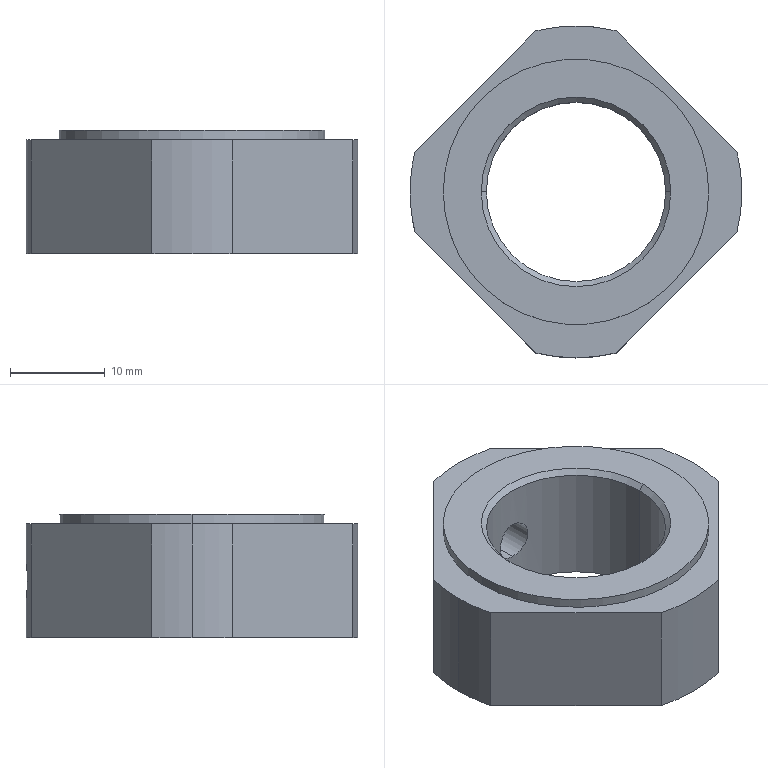Part | STEP file | BKN26-M20 | 1 solid | 20 faces | box 35 x 35 x 13 mm | volume 6926 mm3 | cylinder 11 | plane 7 | cone 2 | commonest cylinder face diameters 35 x5 4.134 x2 18.917 x2 28 x2
STEP:
#1=CARTESIAN_POINT('',(9.458,0.,12.459));
#2=VERTEX_POINT('',#1);
#3=CARTESIAN_POINT('',(-9.458,0.,12.459));
#4=VERTEX_POINT('',#3);
#5=CARTESIAN_POINT('',(0.,0.,12.459));
#6=DIRECTION('',(0.,0.,-1.));
#7=DIRECTION('',(-1.,0.,0.));
#8=AXIS2_PLACEMENT_3D('',#5,#6,#7);
#9=CIRCLE('',#8,9.458);
#10=EDGE_CURVE('',#2,#4,#9,.T.);
#11=ORIENTED_EDGE('',*,*,#10,.T.);
#12=CARTESIAN_POINT('',(-10.,0.,13.));
#13=VERTEX_POINT('',#12);
#14=CARTESIAN_POINT('',(-10.,0.,13.));
#15=DIRECTION('',(-0.7071,0.,0.7071));
#16=VECTOR('',#15,1000.);
#17=LINE('',#14,#16);
#18=EDGE_CURVE('',#4,#13,#17,.T.);
#19=ORIENTED_EDGE('',*,*,#18,.T.);
#20=CARTESIAN_POINT('',(10.,0.,13.));
#21=VERTEX_POINT('',#20);
#22=CARTESIAN_POINT('',(0.,0.,13.));
#23=DIRECTION('',(0.,0.,-1.));
#24=DIRECTION('',(-1.,0.,0.));
#25=AXIS2_PLACEMENT_3D('',#22,#23,#24);
#26=CIRCLE('',#25,10.);
#27=EDGE_CURVE('',#21,#13,#26,.T.);
#28=ORIENTED_EDGE('',*,*,#27,.F.);
#29=CARTESIAN_POINT('',(10.,0.,13.));
#30=DIRECTION('',(0.7071,0.,0.7071));
#31=VECTOR('',#30,1000.);
#32=LINE('',#29,#31);
#33=EDGE_CURVE('',#2,#21,#32,.T.);
#34=ORIENTED_EDGE('',*,*,#33,.F.);
#35=EDGE_LOOP('',(#11,#19,#28,#34));
#36=FACE_OUTER_BOUND('',#35,.T.);
#37=CARTESIAN_POINT('',(0.,0.,13.));
#38=DIRECTION('',(0.,0.,1.));
#39=DIRECTION('',(1.,0.,0.));
#40=AXIS2_PLACEMENT_3D('',#37,#38,#39);
#41=CONICAL_SURFACE('',#40,10.,0.7854);
#42=ADVANCED_FACE('',(#36),#41,.F.);
#43=CARTESIAN_POINT('',(14.,0.,13.));
#44=VERTEX_POINT('',#43);
#45=CARTESIAN_POINT('',(-14.,0.,13.));
#46=VERTEX_POINT('',#45);
#47=CARTESIAN_POINT('',(0.,0.,13.));
#48=DIRECTION('',(0.,0.,1.));
#49=DIRECTION('',(1.,0.,0.));
#50=AXIS2_PLACEMENT_3D('',#47,#48,#49);
#51=CIRCLE('',#50,14.);
#52=EDGE_CURVE('',#44,#46,#51,.T.);
#53=ORIENTED_EDGE('',*,*,#52,.F.);
#54=CARTESIAN_POINT('',(14.,0.,12.));
#55=VERTEX_POINT('',#54);
#56=CARTESIAN_POINT('',(14.,0.,13.));
#57=DIRECTION('',(0.,0.,-1.));
#58=VECTOR('',#57,1000.);
#59=LINE('',#56,#58);
#60=EDGE_CURVE('',#44,#55,#59,.T.);
#61=ORIENTED_EDGE('',*,*,#60,.T.);
#62=CARTESIAN_POINT('',(-14.,0.,12.));
#63=VERTEX_POINT('',#62);
#64=CARTESIAN_POINT('',(0.,0.,12.));
#65=DIRECTION('',(0.,0.,-1.));
#66=DIRECTION('',(1.,0.,0.));
#67=AXIS2_PLACEMENT_3D('',#64,#65,#66);
#68=CIRCLE('',#67,14.);
#69=EDGE_CURVE('',#63,#55,#68,.T.);
#70=ORIENTED_EDGE('',*,*,#69,.F.);
#71=CARTESIAN_POINT('',(-14.,0.,13.));
#72=DIRECTION('',(0.,0.,-1.));
#73=VECTOR('',#72,1000.);
#74=LINE('',#71,#73);
#75=EDGE_CURVE('',#46,#63,#74,.T.);
#76=ORIENTED_EDGE('',*,*,#75,.F.);
#77=EDGE_LOOP('',(#53,#61,#70,#76));
#78=FACE_OUTER_BOUND('',#77,.T.);
#79=CARTESIAN_POINT('',(0.,0.,13.));
#80=DIRECTION('',(0.,0.,-1.));
#81=DIRECTION('',(-1.,0.,0.));
#82=AXIS2_PLACEMENT_3D('',#79,#80,#81);
#83=CYLINDRICAL_SURFACE('',#82,14.);
#84=ADVANCED_FACE('',(#78),#83,.T.);
#85=CARTESIAN_POINT('',(-17.5,0.,12.));
#86=VERTEX_POINT('',#85);
#87=CARTESIAN_POINT('',(-16.98,-4.233,12.));
#88=VERTEX_POINT('',#87);
#89=CARTESIAN_POINT('',(0.,0.,12.));
#90=DIRECTION('',(0.,0.,1.));
#91=DIRECTION('',(-0.9703,0.2419,0.));
#92=AXIS2_PLACEMENT_3D('',#89,#90,#91);
#93=CIRCLE('',#92,17.5);
#94=EDGE_CURVE('',#86,#88,#93,.T.);
#95=ORIENTED_EDGE('',*,*,#94,.F.);
#96=CARTESIAN_POINT('',(-17.5,0.,0.));
#97=VERTEX_POINT('',#96);
#98=CARTESIAN_POINT('',(-17.5,0.,12.));
#99=DIRECTION('',(0.,0.,-1.));
#100=VECTOR('',#99,1000.);
#101=LINE('',#98,#100);
#102=EDGE_CURVE('',#86,#97,#101,.T.);
#103=ORIENTED_EDGE('',*,*,#102,.T.);
#104=CARTESIAN_POINT('',(-16.98,-4.233,0.));
#105=VERTEX_POINT('',#104);
#106=CARTESIAN_POINT('',(0.,0.,0.));
#107=DIRECTION('',(0.,0.,1.));
#108=DIRECTION('',(-0.9703,0.2419,0.));
#109=AXIS2_PLACEMENT_3D('',#106,#107,#108);
#110=CIRCLE('',#109,17.5);
#111=EDGE_CURVE('',#97,#105,#110,.T.);
#112=ORIENTED_EDGE('',*,*,#111,.T.);
#113=CARTESIAN_POINT('',(-16.98,-4.233,12.));
#114=DIRECTION('',(0.,0.,-1.));
#115=VECTOR('',#114,1000.);
#116=LINE('',#113,#115);
#117=EDGE_CURVE('',#88,#105,#116,.T.);
#118=ORIENTED_EDGE('',*,*,#117,.F.);
#119=EDGE_LOOP('',(#95,#103,#112,#118));
#120=FACE_OUTER_BOUND('',#119,.T.);
#121=CARTESIAN_POINT('',(0.,0.,12.));
#122=DIRECTION('',(0.,0.,-1.));
#123=DIRECTION('',(-1.,0.,0.));
#124=AXIS2_PLACEMENT_3D('',#121,#122,#123);
#125=CYLINDRICAL_SURFACE('',#124,17.5);
#126=ADVANCED_FACE('',(#120),#125,.T.);
#127=ORIENTED_EDGE('',*,*,#10,.F.);
#128=CARTESIAN_POINT('',(9.458,0.,0.));
#129=VERTEX_POINT('',#128);
#130=CARTESIAN_POINT('',(9.458,0.,0.));
#131=DIRECTION('',(0.,0.,-1.));
#132=VECTOR('',#131,1000.);
#133=LINE('',#130,#132);
#134=EDGE_CURVE('',#2,#129,#133,.T.);
#135=ORIENTED_EDGE('',*,*,#134,.T.);
#136=CARTESIAN_POINT('',(-9.458,0.,0.));
#137=VERTEX_POINT('',#136);
#138=CARTESIAN_POINT('',(0.,0.,0.));
#139=DIRECTION('',(0.,0.,-1.));
#140=DIRECTION('',(-1.,0.,0.));
#141=AXIS2_PLACEMENT_3D('',#138,#139,#140);
#142=CIRCLE('',#141,9.458);
#143=EDGE_CURVE('',#129,#137,#142,.T.);
#144=ORIENTED_EDGE('',*,*,#143,.T.);
#145=CARTESIAN_POINT('',(-9.458,0.,0.));
#146=DIRECTION('',(0.,0.,-1.));
#147=VECTOR('',#146,1000.);
#148=LINE('',#145,#147);
#149=EDGE_CURVE('',#4,#137,#148,.T.);
#150=ORIENTED_EDGE('',*,*,#149,.F.);
#151=EDGE_LOOP('',(#127,#135,#144,#150));
#152=FACE_OUTER_BOUND('',#151,.T.);
#153=CARTESIAN_POINT('',(0.,0.,0.));
#154=DIRECTION('',(0.,0.,-1.));
#155=DIRECTION('',(-1.,0.,0.));
#156=AXIS2_PLACEMENT_3D('',#153,#154,#155);
#157=CYLINDRICAL_SURFACE('',#156,9.458);
#158=ADVANCED_FACE('',(#152),#157,.F.);
#159=CARTESIAN_POINT('',(0.,17.5,3.933));
#160=VERTEX_POINT('',#159);
#161=CARTESIAN_POINT('',(-0.000000115,17.5,8.067));
#162=VERTEX_POINT('',#161);
#163=CARTESIAN_POINT('',(0.,17.5,3.933));
#164=CARTESIAN_POINT('',(-0.2708,17.5,3.933));
#165=CARTESIAN_POINT('',(-0.5415,17.493,3.987));
#166=CARTESIAN_POINT('',(-1.041,17.471,4.194));
#167=CARTESIAN_POINT('',(-1.27,17.455,4.347));
#168=CARTESIAN_POINT('',(-1.653,17.423,4.73));
#169=CARTESIAN_POINT('',(-1.806,17.407,4.959));
#170=CARTESIAN_POINT('',(-2.013,17.384,5.459));
#171=CARTESIAN_POINT('',(-2.067,17.378,5.729));
#172=CARTESIAN_POINT('',(-2.067,17.377,6.271));
#173=CARTESIAN_POINT('',(-2.013,17.384,6.541));
#174=CARTESIAN_POINT('',(-1.806,17.407,7.041));
#175=CARTESIAN_POINT('',(-1.653,17.423,7.27));
#176=CARTESIAN_POINT('',(-1.27,17.455,7.653));
#177=CARTESIAN_POINT('',(-1.041,17.471,7.806));
#178=CARTESIAN_POINT('',(-0.5414,17.493,8.013));
#179=CARTESIAN_POINT('',(-0.2708,17.5,8.067));
#180=CARTESIAN_POINT('',(-0.000000115,17.5,8.067));
#181=B_SPLINE_CURVE_WITH_KNOTS('',3,(#163,#164,#165,#166,#167,#168,#169,#170,#171,#172,#173,#174,#175,#176,#177,#178,#179,#180),.UNSPECIFIED.,.F.,.F.,(4,2,2,2,2,2,2,2,4),(0.,0.8086,1.617,2.426,3.234,4.043,4.851,5.66,6.469),.UNSPECIFIED.);
#182=EDGE_CURVE('',#160,#162,#181,.T.);
#183=ORIENTED_EDGE('',*,*,#182,.T.);
#184=CARTESIAN_POINT('',(-0.000000086,9.458,8.067));
#185=VERTEX_POINT('',#184);
#186=CARTESIAN_POINT('',(0.,9.,8.067));
#187=DIRECTION('',(0.,-1.,0.));
#188=VECTOR('',#187,1000.);
#189=LINE('',#186,#188);
#190=EDGE_CURVE('',#162,#185,#189,.T.);
#191=ORIENTED_EDGE('',*,*,#190,.T.);
#192=CARTESIAN_POINT('',(0.,9.458,3.933));
#193=VERTEX_POINT('',#192);
#194=CARTESIAN_POINT('',(0.,9.458,3.933));
#195=CARTESIAN_POINT('',(-0.137,9.458,3.933));
#196=CARTESIAN_POINT('',(-0.2717,9.456,3.946));
#197=CARTESIAN_POINT('',(-0.5365,9.444,3.999));
#198=CARTESIAN_POINT('',(-0.6679,9.436,4.039));
#199=CARTESIAN_POINT('',(-0.9182,9.415,4.143));
#200=CARTESIAN_POINT('',(-1.037,9.402,4.206));
#201=CARTESIAN_POINT('',(-1.261,9.375,4.357));
#202=CARTESIAN_POINT('',(-1.367,9.36,4.444));
#203=CARTESIAN_POINT('',(-1.652,9.315,4.729));
#204=CARTESIAN_POINT('',(-1.806,9.285,4.959));
#205=CARTESIAN_POINT('',(-2.012,9.243,5.456));
#206=CARTESIAN_POINT('',(-2.067,9.23,5.729));
#207=CARTESIAN_POINT('',(-2.067,9.23,6.134));
#208=CARTESIAN_POINT('',(-2.054,9.233,6.272));
#209=CARTESIAN_POINT('',(-2.001,9.245,6.537));
#210=CARTESIAN_POINT('',(-1.961,9.253,6.666));
#211=CARTESIAN_POINT('',(-1.805,9.285,7.043));
#212=CARTESIAN_POINT('',(-1.653,9.315,7.27));
#213=CARTESIAN_POINT('',(-1.365,9.36,7.558));
#214=CARTESIAN_POINT('',(-1.262,9.375,7.643));
#215=CARTESIAN_POINT('',(-1.038,9.402,7.793));
#216=CARTESIAN_POINT('',(-0.9169,9.415,7.857));
#217=CARTESIAN_POINT('',(-0.6672,9.436,7.961));
#218=CARTESIAN_POINT('',(-0.5383,9.444,8.001));
#219=CARTESIAN_POINT('',(-0.2723,9.456,8.053));
#220=CARTESIAN_POINT('',(-0.1352,9.458,8.067));
#221=CARTESIAN_POINT('',(-0.000000086,9.458,8.067));
#222=B_SPLINE_CURVE_WITH_KNOTS('',3,(#194,#195,#196,#197,#198,#199,#200,#201,#202,#203,#204,#205,#206,#207,#208,#209,#210,#211,#212,#213,#214,#215,#216,#217,#218,#219,#220,#221),.UNSPECIFIED.,.F.,.F.,(4,2,2,2,2,2,2,2,2,2,2,2,2,4),(0.,0.4051,0.8102,1.215,1.62,2.431,3.241,3.646,4.051,4.861,5.267,5.672,6.077,6.482),.UNSPECIFIED.);
#223=EDGE_CURVE('',#193,#185,#222,.T.);
#224=ORIENTED_EDGE('',*,*,#223,.F.);
#225=CARTESIAN_POINT('',(0.,9.,3.933));
#226=DIRECTION('',(0.,-1.,0.));
#227=VECTOR('',#226,1000.);
#228=LINE('',#225,#227);
#229=EDGE_CURVE('',#160,#193,#228,.T.);
#230=ORIENTED_EDGE('',*,*,#229,.F.);
#231=EDGE_LOOP('',(#183,#191,#224,#230));
#232=FACE_OUTER_BOUND('',#231,.T.);
#233=CARTESIAN_POINT('',(0.,9.,6.));
#234=DIRECTION('',(0.,-1.,0.));
#235=DIRECTION('',(0.,0.,-1.));
#236=AXIS2_PLACEMENT_3D('',#233,#234,#235);
#237=CYLINDRICAL_SURFACE('',#236,2.067);
#238=ADVANCED_FACE('',(#232),#237,.F.);
#239=CARTESIAN_POINT('',(4.233,16.98,0.));
#240=VERTEX_POINT('',#239);
#241=CARTESIAN_POINT('',(-4.233,16.98,0.));
#242=VERTEX_POINT('',#241);
#243=CARTESIAN_POINT('',(0.,0.,0.));
#244=DIRECTION('',(0.,0.,1.));
#245=DIRECTION('',(0.2419,0.9703,0.));
#246=AXIS2_PLACEMENT_3D('',#243,#244,#245);
#247=CIRCLE('',#246,17.5);
#248=EDGE_CURVE('',#240,#242,#247,.T.);
#249=ORIENTED_EDGE('',*,*,#248,.T.);
#250=CARTESIAN_POINT('',(-4.233,16.98,12.));
#251=VERTEX_POINT('',#250);
#252=CARTESIAN_POINT('',(-4.233,16.98,12.));
#253=DIRECTION('',(0.,0.,-1.));
#254=VECTOR('',#253,1000.);
#255=LINE('',#252,#254);
#256=EDGE_CURVE('',#251,#242,#255,.T.);
#257=ORIENTED_EDGE('',*,*,#256,.F.);
#258=CARTESIAN_POINT('',(4.233,16.98,12.));
#259=VERTEX_POINT('',#258);
#260=CARTESIAN_POINT('',(0.,0.,12.));
#261=DIRECTION('',(0.,0.,1.));
#262=DIRECTION('',(0.2419,0.9703,0.));
#263=AXIS2_PLACEMENT_3D('',#260,#261,#262);
#264=CIRCLE('',#263,17.5);
#265=EDGE_CURVE('',#259,#251,#264,.T.);
#266=ORIENTED_EDGE('',*,*,#265,.F.);
#267=CARTESIAN_POINT('',(4.233,16.98,12.));
#268=DIRECTION('',(0.,0.,-1.));
#269=VECTOR('',#268,1000.);
#270=LINE('',#267,#269);
#271=EDGE_CURVE('',#259,#240,#270,.T.);
#272=ORIENTED_EDGE('',*,*,#271,.T.);
#273=EDGE_LOOP('',(#249,#257,#266,#272));
#274=FACE_OUTER_BOUND('',#273,.T.);
#275=ORIENTED_EDGE('',*,*,#182,.F.);
#276=CARTESIAN_POINT('',(-0.000000115,17.5,8.067));
#277=CARTESIAN_POINT('',(0.2707,17.5,8.067));
#278=CARTESIAN_POINT('',(0.5413,17.493,8.013));
#279=CARTESIAN_POINT('',(1.041,17.471,7.806));
#280=CARTESIAN_POINT('',(1.27,17.455,7.653));
#281=CARTESIAN_POINT('',(1.652,17.423,7.271));
#282=CARTESIAN_POINT('',(1.805,17.407,7.042));
#283=CARTESIAN_POINT('',(2.013,17.384,6.542));
#284=CARTESIAN_POINT('',(2.067,17.378,6.272));
#285=CARTESIAN_POINT('',(2.067,17.377,5.731));
#286=CARTESIAN_POINT('',(2.013,17.384,5.46));
#287=CARTESIAN_POINT('',(1.807,17.407,4.96));
#288=CARTESIAN_POINT('',(1.654,17.423,4.731));
#289=CARTESIAN_POINT('',(1.272,17.455,4.348));
#290=CARTESIAN_POINT('',(1.043,17.471,4.195));
#291=CARTESIAN_POINT('',(0.5441,17.493,3.988));
#292=CARTESIAN_POINT('',(0.2722,17.5,3.933));
#293=CARTESIAN_POINT('',(0.,17.5,3.933));
#294=B_SPLINE_CURVE_WITH_KNOTS('',3,(#276,#277,#278,#279,#280,#281,#282,#283,#284,#285,#286,#287,#288,#289,#290,#291,#292,#293),.UNSPECIFIED.,.F.,.F.,(4,2,2,2,2,2,2,2,4),(6.469,7.277,8.085,8.893,9.702,10.51,11.318,12.126,12.935),.UNSPECIFIED.);
#295=EDGE_CURVE('',#162,#160,#294,.T.);
#296=ORIENTED_EDGE('',*,*,#295,.F.);
#297=EDGE_LOOP('',(#275,#296));
#298=FACE_BOUND('',#297,.T.);
#299=CARTESIAN_POINT('',(0.,0.,12.));
#300=DIRECTION('',(0.,0.,-1.));
#301=DIRECTION('',(-1.,0.,0.));
#302=AXIS2_PLACEMENT_3D('',#299,#300,#301);
#303=CYLINDRICAL_SURFACE('',#302,17.5);
#304=ADVANCED_FACE('',(#274,#298),#303,.T.);
#305=CARTESIAN_POINT('',(0.,0.,0.));
#306=DIRECTION('',(0.,0.,-1.));
#307=DIRECTION('',(-1.,0.,0.));
#308=AXIS2_PLACEMENT_3D('',#305,#306,#307);
#309=CIRCLE('',#308,9.458);
#310=EDGE_CURVE('',#137,#129,#309,.T.);
#311=ORIENTED_EDGE('',*,*,#310,.F.);
#312=ORIENTED_EDGE('',*,*,#143,.F.);
#313=EDGE_LOOP('',(#311,#312));
#314=FACE_BOUND('',#313,.T.);
#315=CARTESIAN_POINT('',(-16.98,4.233,0.));
#316=VERTEX_POINT('',#315);
#317=CARTESIAN_POINT('',(-4.233,16.98,0.));
#318=DIRECTION('',(-0.7071,-0.7071,0.));
#319=VECTOR('',#318,1000.);
#320=LINE('',#317,#319);
#321=EDGE_CURVE('',#242,#316,#320,.T.);
#322=ORIENTED_EDGE('',*,*,#321,.F.);
#323=ORIENTED_EDGE('',*,*,#248,.F.);
#324=CARTESIAN_POINT('',(16.98,4.233,0.));
#325=VERTEX_POINT('',#324);
#326=CARTESIAN_POINT('',(16.98,4.233,0.));
#327=DIRECTION('',(-0.7071,0.7071,0.));
#328=VECTOR('',#327,1000.);
#329=LINE('',#326,#328);
#330=EDGE_CURVE('',#325,#240,#329,.T.);
#331=ORIENTED_EDGE('',*,*,#330,.F.);
#332=CARTESIAN_POINT('',(16.98,-4.233,0.));
#333=VERTEX_POINT('',#332);
#334=CARTESIAN_POINT('',(0.,0.,0.));
#335=DIRECTION('',(0.,0.,1.));
#336=DIRECTION('',(0.9703,-0.2419,0.));
#337=AXIS2_PLACEMENT_3D('',#334,#335,#336);
#338=CIRCLE('',#337,17.5);
#339=EDGE_CURVE('',#333,#325,#338,.T.);
#340=ORIENTED_EDGE('',*,*,#339,.F.);
#341=CARTESIAN_POINT('',(4.233,-16.98,0.));
#342=VERTEX_POINT('',#341);
#343=CARTESIAN_POINT('',(4.233,-16.98,0.));
#344=DIRECTION('',(0.7071,0.7071,0.));
#345=VECTOR('',#344,1000.);
#346=LINE('',#343,#345);
#347=EDGE_CURVE('',#342,#333,#346,.T.);
#348=ORIENTED_EDGE('',*,*,#347,.F.);
#349=CARTESIAN_POINT('',(-4.233,-16.98,0.));
#350=VERTEX_POINT('',#349);
#351=CARTESIAN_POINT('',(0.,0.,0.));
#352=DIRECTION('',(0.,0.,1.));
#353=DIRECTION('',(-0.2419,-0.9703,0.));
#354=AXIS2_PLACEMENT_3D('',#351,#352,#353);
#355=CIRCLE('',#354,17.5);
#356=EDGE_CURVE('',#350,#342,#355,.T.);
#357=ORIENTED_EDGE('',*,*,#356,.F.);
#358=CARTESIAN_POINT('',(-16.98,-4.233,0.));
#359=DIRECTION('',(0.7071,-0.7071,0.));
#360=VECTOR('',#359,1000.);
#361=LINE('',#358,#360);
#362=EDGE_CURVE('',#105,#350,#361,.T.);
#363=ORIENTED_EDGE('',*,*,#362,.F.);
#364=ORIENTED_EDGE('',*,*,#111,.F.);
#365=CARTESIAN_POINT('',(0.,0.,0.));
#366=DIRECTION('',(0.,0.,1.));
#367=DIRECTION('',(-0.9703,0.2419,0.));
#368=AXIS2_PLACEMENT_3D('',#365,#366,#367);
#369=CIRCLE('',#368,17.5);
#370=EDGE_CURVE('',#316,#97,#369,.T.);
#371=ORIENTED_EDGE('',*,*,#370,.F.);
#372=EDGE_LOOP('',(#322,#323,#331,#340,#348,#357,#363,#364,#371));
#373=FACE_OUTER_BOUND('',#372,.T.);
#374=CARTESIAN_POINT('',(0.,0.,0.));
#375=DIRECTION('',(0.,0.,1.));
#376=DIRECTION('',(1.,0.,0.));
#377=AXIS2_PLACEMENT_3D('',#374,#375,#376);
#378=PLANE('',#377);
#379=ADVANCED_FACE('',(#314,#373),#378,.F.);
#380=ORIENTED_EDGE('',*,*,#321,.T.);
#381=CARTESIAN_POINT('',(-16.98,4.233,12.));
#382=VERTEX_POINT('',#381);
#383=CARTESIAN_POINT('',(-16.98,4.233,12.));
#384=DIRECTION('',(0.,0.,-1.));
#385=VECTOR('',#384,1000.);
#386=LINE('',#383,#385);
#387=EDGE_CURVE('',#382,#316,#386,.T.);
#388=ORIENTED_EDGE('',*,*,#387,.F.);
#389=CARTESIAN_POINT('',(-4.233,16.98,12.));
#390=DIRECTION('',(-0.7071,-0.7071,0.));
#391=VECTOR('',#390,1000.);
#392=LINE('',#389,#391);
#393=EDGE_CURVE('',#251,#382,#392,.T.);
#394=ORIENTED_EDGE('',*,*,#393,.F.);
#395=ORIENTED_EDGE('',*,*,#256,.T.);
#396=EDGE_LOOP('',(#380,#388,#394,#395));
#397=FACE_OUTER_BOUND('',#396,.T.);
#398=CARTESIAN_POINT('',(-4.233,16.98,12.));
#399=DIRECTION('',(0.7071,-0.7071,0.));
#400=DIRECTION('',(0.7071,0.7071,0.));
#401=AXIS2_PLACEMENT_3D('',#398,#399,#400);
#402=PLANE('',#401);
#403=ADVANCED_FACE('',(#397),#402,.F.);
#404=ORIENTED_EDGE('',*,*,#69,.T.);
#405=CARTESIAN_POINT('',(0.,0.,12.));
#406=DIRECTION('',(0.,0.,-1.));
#407=DIRECTION('',(1.,0.,0.));
#408=AXIS2_PLACEMENT_3D('',#405,#406,#407);
#409=CIRCLE('',#408,14.);
#410=EDGE_CURVE('',#55,#63,#409,.T.);
#411=ORIENTED_EDGE('',*,*,#410,.T.);
#412=EDGE_LOOP('',(#404,#411));
#413=FACE_BOUND('',#412,.T.);
#414=ORIENTED_EDGE('',*,*,#393,.T.);
#415=CARTESIAN_POINT('',(0.,0.,12.));
#416=DIRECTION('',(0.,0.,1.));
#417=DIRECTION('',(-0.9703,0.2419,0.));
#418=AXIS2_PLACEMENT_3D('',#415,#416,#417);
#419=CIRCLE('',#418,17.5);
#420=EDGE_CURVE('',#382,#86,#419,.T.);
#421=ORIENTED_EDGE('',*,*,#420,.T.);
#422=ORIENTED_EDGE('',*,*,#94,.T.);
#423=CARTESIAN_POINT('',(-4.233,-16.98,12.));
#424=VERTEX_POINT('',#423);
#425=CARTESIAN_POINT('',(-16.98,-4.233,12.));
#426=DIRECTION('',(0.7071,-0.7071,0.));
#427=VECTOR('',#426,1000.);
#428=LINE('',#425,#427);
#429=EDGE_CURVE('',#88,#424,#428,.T.);
#430=ORIENTED_EDGE('',*,*,#429,.T.);
#431=CARTESIAN_POINT('',(4.233,-16.98,12.));
#432=VERTEX_POINT('',#431);
#433=CARTESIAN_POINT('',(0.,0.,12.));
#434=DIRECTION('',(0.,0.,1.));
#435=DIRECTION('',(-0.2419,-0.9703,0.));
#436=AXIS2_PLACEMENT_3D('',#433,#434,#435);
#437=CIRCLE('',#436,17.5);
#438=EDGE_CURVE('',#424,#432,#437,.T.);
#439=ORIENTED_EDGE('',*,*,#438,.T.);
#440=CARTESIAN_POINT('',(16.98,-4.233,12.));
#441=VERTEX_POINT('',#440);
#442=CARTESIAN_POINT('',(4.233,-16.98,12.));
#443=DIRECTION('',(0.7071,0.7071,0.));
#444=VECTOR('',#443,1000.);
#445=LINE('',#442,#444);
#446=EDGE_CURVE('',#432,#441,#445,.T.);
#447=ORIENTED_EDGE('',*,*,#446,.T.);
#448=CARTESIAN_POINT('',(16.98,4.233,12.));
#449=VERTEX_POINT('',#448);
#450=CARTESIAN_POINT('',(0.,0.,12.));
#451=DIRECTION('',(0.,0.,1.));
#452=DIRECTION('',(0.9703,-0.2419,0.));
#453=AXIS2_PLACEMENT_3D('',#450,#451,#452);
#454=CIRCLE('',#453,17.5);
#455=EDGE_CURVE('',#441,#449,#454,.T.);
#456=ORIENTED_EDGE('',*,*,#455,.T.);
#457=CARTESIAN_POINT('',(16.98,4.233,12.));
#458=DIRECTION('',(-0.7071,0.7071,0.));
#459=VECTOR('',#458,1000.);
#460=LINE('',#457,#459);
#461=EDGE_CURVE('',#449,#259,#460,.T.);
#462=ORIENTED_EDGE('',*,*,#461,.T.);
#463=ORIENTED_EDGE('',*,*,#265,.T.);
#464=EDGE_LOOP('',(#414,#421,#422,#430,#439,#447,#456,#462,#463));
#465=FACE_OUTER_BOUND('',#464,.T.);
#466=CARTESIAN_POINT('',(0.,0.,12.));
#467=DIRECTION('',(0.,0.,1.));
#468=DIRECTION('',(1.,0.,0.));
#469=AXIS2_PLACEMENT_3D('',#466,#467,#468);
#470=PLANE('',#469);
#471=ADVANCED_FACE('',(#413,#465),#470,.T.);
#472=ORIENTED_EDGE('',*,*,#330,.T.);
#473=ORIENTED_EDGE('',*,*,#271,.F.);
#474=ORIENTED_EDGE('',*,*,#461,.F.);
#475=CARTESIAN_POINT('',(16.98,4.233,12.));
#476=DIRECTION('',(0.,0.,-1.));
#477=VECTOR('',#476,1000.);
#478=LINE('',#475,#477);
#479=EDGE_CURVE('',#449,#325,#478,.T.);
#480=ORIENTED_EDGE('',*,*,#479,.T.);
#481=EDGE_LOOP('',(#472,#473,#474,#480));
#482=FACE_OUTER_BOUND('',#481,.T.);
#483=CARTESIAN_POINT('',(16.98,4.233,12.));
#484=DIRECTION('',(-0.7071,-0.7071,0.));
#485=DIRECTION('',(0.7071,-0.7071,0.));
#486=AXIS2_PLACEMENT_3D('',#483,#484,#485);
#487=PLANE('',#486);
#488=ADVANCED_FACE('',(#482),#487,.F.);
#489=ORIENTED_EDGE('',*,*,#190,.F.);
#490=ORIENTED_EDGE('',*,*,#295,.T.);
#491=ORIENTED_EDGE('',*,*,#229,.T.);
#492=CARTESIAN_POINT('',(-0.000000086,9.458,8.067));
#493=CARTESIAN_POINT('',(0.2702,9.459,8.067));
#494=CARTESIAN_POINT('',(0.543,9.446,8.013));
#495=CARTESIAN_POINT('',(0.9163,9.415,7.858));
#496=CARTESIAN_POINT('',(1.037,9.402,7.793));
#497=CARTESIAN_POINT('',(1.262,9.375,7.643));
#498=CARTESIAN_POINT('',(1.366,9.36,7.558));
#499=CARTESIAN_POINT('',(1.556,9.33,7.367));
#500=CARTESIAN_POINT('',(1.643,9.315,7.261));
#501=CARTESIAN_POINT('',(1.793,9.287,7.038));
#502=CARTESIAN_POINT('',(1.856,9.275,6.919));
#503=CARTESIAN_POINT('',(2.013,9.242,6.543));
#504=CARTESIAN_POINT('',(2.067,9.23,6.274));
#505=CARTESIAN_POINT('',(2.067,9.23,5.864));
#506=CARTESIAN_POINT('',(2.054,9.233,5.73));
#507=CARTESIAN_POINT('',(2.001,9.244,5.465));
#508=CARTESIAN_POINT('',(1.961,9.253,5.333));
#509=CARTESIAN_POINT('',(1.858,9.274,5.083));
#510=CARTESIAN_POINT('',(1.794,9.287,4.965));
#511=CARTESIAN_POINT('',(1.644,9.315,4.74));
#512=CARTESIAN_POINT('',(1.557,9.33,4.634));
#513=CARTESIAN_POINT('',(1.273,9.374,4.349));
#514=CARTESIAN_POINT('',(1.043,9.404,4.195));
#515=CARTESIAN_POINT('',(0.6701,9.436,4.04));
#516=CARTESIAN_POINT('',(0.5388,9.444,4.));
#517=CARTESIAN_POINT('',(0.2721,9.456,3.946));
#518=CARTESIAN_POINT('',(0.1369,9.458,3.933));
#519=CARTESIAN_POINT('',(0.,9.458,3.933));
#520=B_SPLINE_CURVE_WITH_KNOTS('',3,(#492,#493,#494,#495,#496,#497,#498,#499,#500,#501,#502,#503,#504,#505,#506,#507,#508,#509,#510,#511,#512,#513,#514,#515,#516,#517,#518,#519),.UNSPECIFIED.,.F.,.F.,(4,2,2,2,2,2,2,2,2,2,2,2,2,4),(6.482,7.292,7.697,8.102,8.507,8.912,9.722,10.127,10.532,10.937,11.342,12.152,12.557,12.962),.UNSPECIFIED.);
#521=EDGE_CURVE('',#185,#193,#520,.T.);
#522=ORIENTED_EDGE('',*,*,#521,.F.);
#523=EDGE_LOOP('',(#489,#490,#491,#522));
#524=FACE_OUTER_BOUND('',#523,.T.);
#525=CARTESIAN_POINT('',(0.,9.,6.));
#526=DIRECTION('',(0.,-1.,0.));
#527=DIRECTION('',(0.,0.,-1.));
#528=AXIS2_PLACEMENT_3D('',#525,#526,#527);
#529=CYLINDRICAL_SURFACE('',#528,2.067);
#530=ADVANCED_FACE('',(#524),#529,.F.);
#531=ORIENTED_EDGE('',*,*,#134,.F.);
#532=CARTESIAN_POINT('',(0.,0.,12.459));
#533=DIRECTION('',(0.,0.,-1.));
#534=DIRECTION('',(-1.,0.,0.));
#535=AXIS2_PLACEMENT_3D('',#532,#533,#534);
#536=CIRCLE('',#535,9.458);
#537=EDGE_CURVE('',#4,#2,#536,.T.);
#538=ORIENTED_EDGE('',*,*,#537,.F.);
#539=ORIENTED_EDGE('',*,*,#149,.T.);
#540=ORIENTED_EDGE('',*,*,#310,.T.);
#541=EDGE_LOOP('',(#531,#538,#539,#540));
#542=FACE_OUTER_BOUND('',#541,.T.);
#543=ORIENTED_EDGE('',*,*,#223,.T.);
#544=ORIENTED_EDGE('',*,*,#521,.T.);
#545=EDGE_LOOP('',(#543,#544));
#546=FACE_BOUND('',#545,.T.);
#547=CARTESIAN_POINT('',(0.,0.,0.));
#548=DIRECTION('',(0.,0.,-1.));
#549=DIRECTION('',(-1.,0.,0.));
#550=AXIS2_PLACEMENT_3D('',#547,#548,#549);
#551=CYLINDRICAL_SURFACE('',#550,9.458);
#552=ADVANCED_FACE('',(#542,#546),#551,.F.);
#553=ORIENTED_EDGE('',*,*,#339,.T.);
#554=ORIENTED_EDGE('',*,*,#479,.F.);
#555=ORIENTED_EDGE('',*,*,#455,.F.);
#556=CARTESIAN_POINT('',(16.98,-4.233,12.));
#557=DIRECTION('',(0.,0.,-1.));
#558=VECTOR('',#557,1000.);
#559=LINE('',#556,#558);
#560=EDGE_CURVE('',#441,#333,#559,.T.);
#561=ORIENTED_EDGE('',*,*,#560,.T.);
#562=EDGE_LOOP('',(#553,#554,#555,#561));
#563=FACE_OUTER_BOUND('',#562,.T.);
#564=CARTESIAN_POINT('',(0.,0.,12.));
#565=DIRECTION('',(0.,0.,-1.));
#566=DIRECTION('',(-1.,0.,0.));
#567=AXIS2_PLACEMENT_3D('',#564,#565,#566);
#568=CYLINDRICAL_SURFACE('',#567,17.5);
#569=ADVANCED_FACE('',(#563),#568,.T.);
#570=ORIENTED_EDGE('',*,*,#347,.T.);
#571=ORIENTED_EDGE('',*,*,#560,.F.);
#572=ORIENTED_EDGE('',*,*,#446,.F.);
#573=CARTESIAN_POINT('',(4.233,-16.98,12.));
#574=DIRECTION('',(0.,0.,-1.));
#575=VECTOR('',#574,1000.);
#576=LINE('',#573,#575);
#577=EDGE_CURVE('',#432,#342,#576,.T.);
#578=ORIENTED_EDGE('',*,*,#577,.T.);
#579=EDGE_LOOP('',(#570,#571,#572,#578));
#580=FACE_OUTER_BOUND('',#579,.T.);
#581=CARTESIAN_POINT('',(4.233,-16.98,12.));
#582=DIRECTION('',(-0.7071,0.7071,0.));
#583=DIRECTION('',(-0.7071,-0.7071,0.));
#584=AXIS2_PLACEMENT_3D('',#581,#582,#583);
#585=PLANE('',#584);
#586=ADVANCED_FACE('',(#580),#585,.F.);
#587=ORIENTED_EDGE('',*,*,#356,.T.);
#588=ORIENTED_EDGE('',*,*,#577,.F.);
#589=ORIENTED_EDGE('',*,*,#438,.F.);
#590=CARTESIAN_POINT('',(-4.233,-16.98,12.));
#591=DIRECTION('',(0.,0.,-1.));
#592=VECTOR('',#591,1000.);
#593=LINE('',#590,#592);
#594=EDGE_CURVE('',#424,#350,#593,.T.);
#595=ORIENTED_EDGE('',*,*,#594,.T.);
#596=EDGE_LOOP('',(#587,#588,#589,#595));
#597=FACE_OUTER_BOUND('',#596,.T.);
#598=CARTESIAN_POINT('',(0.,0.,12.));
#599=DIRECTION('',(0.,0.,-1.));
#600=DIRECTION('',(-1.,0.,0.));
#601=AXIS2_PLACEMENT_3D('',#598,#599,#600);
#602=CYLINDRICAL_SURFACE('',#601,17.5);
#603=ADVANCED_FACE('',(#597),#602,.T.);
#604=ORIENTED_EDGE('',*,*,#362,.T.);
#605=ORIENTED_EDGE('',*,*,#594,.F.);
#606=ORIENTED_EDGE('',*,*,#429,.F.);
#607=ORIENTED_EDGE('',*,*,#117,.T.);
#608=EDGE_LOOP('',(#604,#605,#606,#607));
#609=FACE_OUTER_BOUND('',#608,.T.);
#610=CARTESIAN_POINT('',(-16.98,-4.233,12.));
#611=DIRECTION('',(0.7071,0.7071,0.));
#612=DIRECTION('',(-0.7071,0.7071,0.));
#613=AXIS2_PLACEMENT_3D('',#610,#611,#612);
#614=PLANE('',#613);
#615=ADVANCED_FACE('',(#609),#614,.F.);
#616=ORIENTED_EDGE('',*,*,#102,.F.);
#617=ORIENTED_EDGE('',*,*,#420,.F.);
#618=ORIENTED_EDGE('',*,*,#387,.T.);
#619=ORIENTED_EDGE('',*,*,#370,.T.);
#620=EDGE_LOOP('',(#616,#617,#618,#619));
#621=FACE_OUTER_BOUND('',#620,.T.);
#622=CARTESIAN_POINT('',(0.,0.,12.));
#623=DIRECTION('',(0.,0.,-1.));
#624=DIRECTION('',(-1.,0.,0.));
#625=AXIS2_PLACEMENT_3D('',#622,#623,#624);
#626=CYLINDRICAL_SURFACE('',#625,17.5);
#627=ADVANCED_FACE('',(#621),#626,.T.);
#628=ORIENTED_EDGE('',*,*,#60,.F.);
#629=CARTESIAN_POINT('',(0.,0.,13.));
#630=DIRECTION('',(0.,0.,1.));
#631=DIRECTION('',(1.,0.,0.));
#632=AXIS2_PLACEMENT_3D('',#629,#630,#631);
#633=CIRCLE('',#632,14.);
#634=EDGE_CURVE('',#46,#44,#633,.T.);
#635=ORIENTED_EDGE('',*,*,#634,.F.);
#636=ORIENTED_EDGE('',*,*,#75,.T.);
#637=ORIENTED_EDGE('',*,*,#410,.F.);
#638=EDGE_LOOP('',(#628,#635,#636,#637));
#639=FACE_OUTER_BOUND('',#638,.T.);
#640=CARTESIAN_POINT('',(0.,0.,13.));
#641=DIRECTION('',(0.,0.,-1.));
#642=DIRECTION('',(-1.,0.,0.));
#643=AXIS2_PLACEMENT_3D('',#640,#641,#642);
#644=CYLINDRICAL_SURFACE('',#643,14.);
#645=ADVANCED_FACE('',(#639),#644,.T.);
#646=ORIENTED_EDGE('',*,*,#18,.F.);
#647=ORIENTED_EDGE('',*,*,#537,.T.);
#648=ORIENTED_EDGE('',*,*,#33,.T.);
#649=CARTESIAN_POINT('',(0.,0.,13.));
#650=DIRECTION('',(0.,0.,-1.));
#651=DIRECTION('',(-1.,0.,0.));
#652=AXIS2_PLACEMENT_3D('',#649,#650,#651);
#653=CIRCLE('',#652,10.);
#654=EDGE_CURVE('',#13,#21,#653,.T.);
#655=ORIENTED_EDGE('',*,*,#654,.F.);
#656=EDGE_LOOP('',(#646,#647,#648,#655));
#657=FACE_OUTER_BOUND('',#656,.T.);
#658=CARTESIAN_POINT('',(0.,0.,13.));
#659=DIRECTION('',(0.,0.,1.));
#660=DIRECTION('',(1.,0.,0.));
#661=AXIS2_PLACEMENT_3D('',#658,#659,#660);
#662=CONICAL_SURFACE('',#661,10.,0.7854);
#663=ADVANCED_FACE('',(#657),#662,.F.);
#664=ORIENTED_EDGE('',*,*,#27,.T.);
#665=ORIENTED_EDGE('',*,*,#654,.T.);
#666=EDGE_LOOP('',(#664,#665));
#667=FACE_BOUND('',#666,.T.);
#668=ORIENTED_EDGE('',*,*,#634,.T.);
#669=ORIENTED_EDGE('',*,*,#52,.T.);
#670=EDGE_LOOP('',(#668,#669));
#671=FACE_OUTER_BOUND('',#670,.T.);
#672=CARTESIAN_POINT('',(0.,0.,13.));
#673=DIRECTION('',(0.,0.,1.));
#674=DIRECTION('',(1.,0.,0.));
#675=AXIS2_PLACEMENT_3D('',#672,#673,#674);
#676=PLANE('',#675);
#677=ADVANCED_FACE('',(#667,#671),#676,.T.);
#678=CLOSED_SHELL('',(#42,#84,#126,#158,#238,#304,#379,#403,#471,#488,#530,#552,#569,#586,#603,#615,#627,#645,#663,#677));
#679=MANIFOLD_SOLID_BREP('',#678);
#680=CARTESIAN_POINT('',(0.,0.,0.));
#681=DIRECTION('',(0.,0.,1.));
#682=DIRECTION('',(1.,0.,0.));
#683=AXIS2_PLACEMENT_3D('',#680,#681,#682);
#684=(LENGTH_UNIT()NAMED_UNIT(*)SI_UNIT(.MILLI.,.METRE.));
#685=UNCERTAINTY_MEASURE_WITH_UNIT(LENGTH_MEASURE(0.00001),#684,'','');
#686=(NAMED_UNIT(*)PLANE_ANGLE_UNIT()SI_UNIT($,.RADIAN.));
#687=(NAMED_UNIT(*)SI_UNIT($,.STERADIAN.)SOLID_ANGLE_UNIT());
#688=(GEOMETRIC_REPRESENTATION_CONTEXT(3)GLOBAL_UNCERTAINTY_ASSIGNED_CONTEXT((#685))GLOBAL_UNIT_ASSIGNED_CONTEXT((#684,#686,#687))REPRESENTATION_CONTEXT('',''));
#689=ADVANCED_BREP_SHAPE_REPRESENTATION('',(#679,#683),#688);